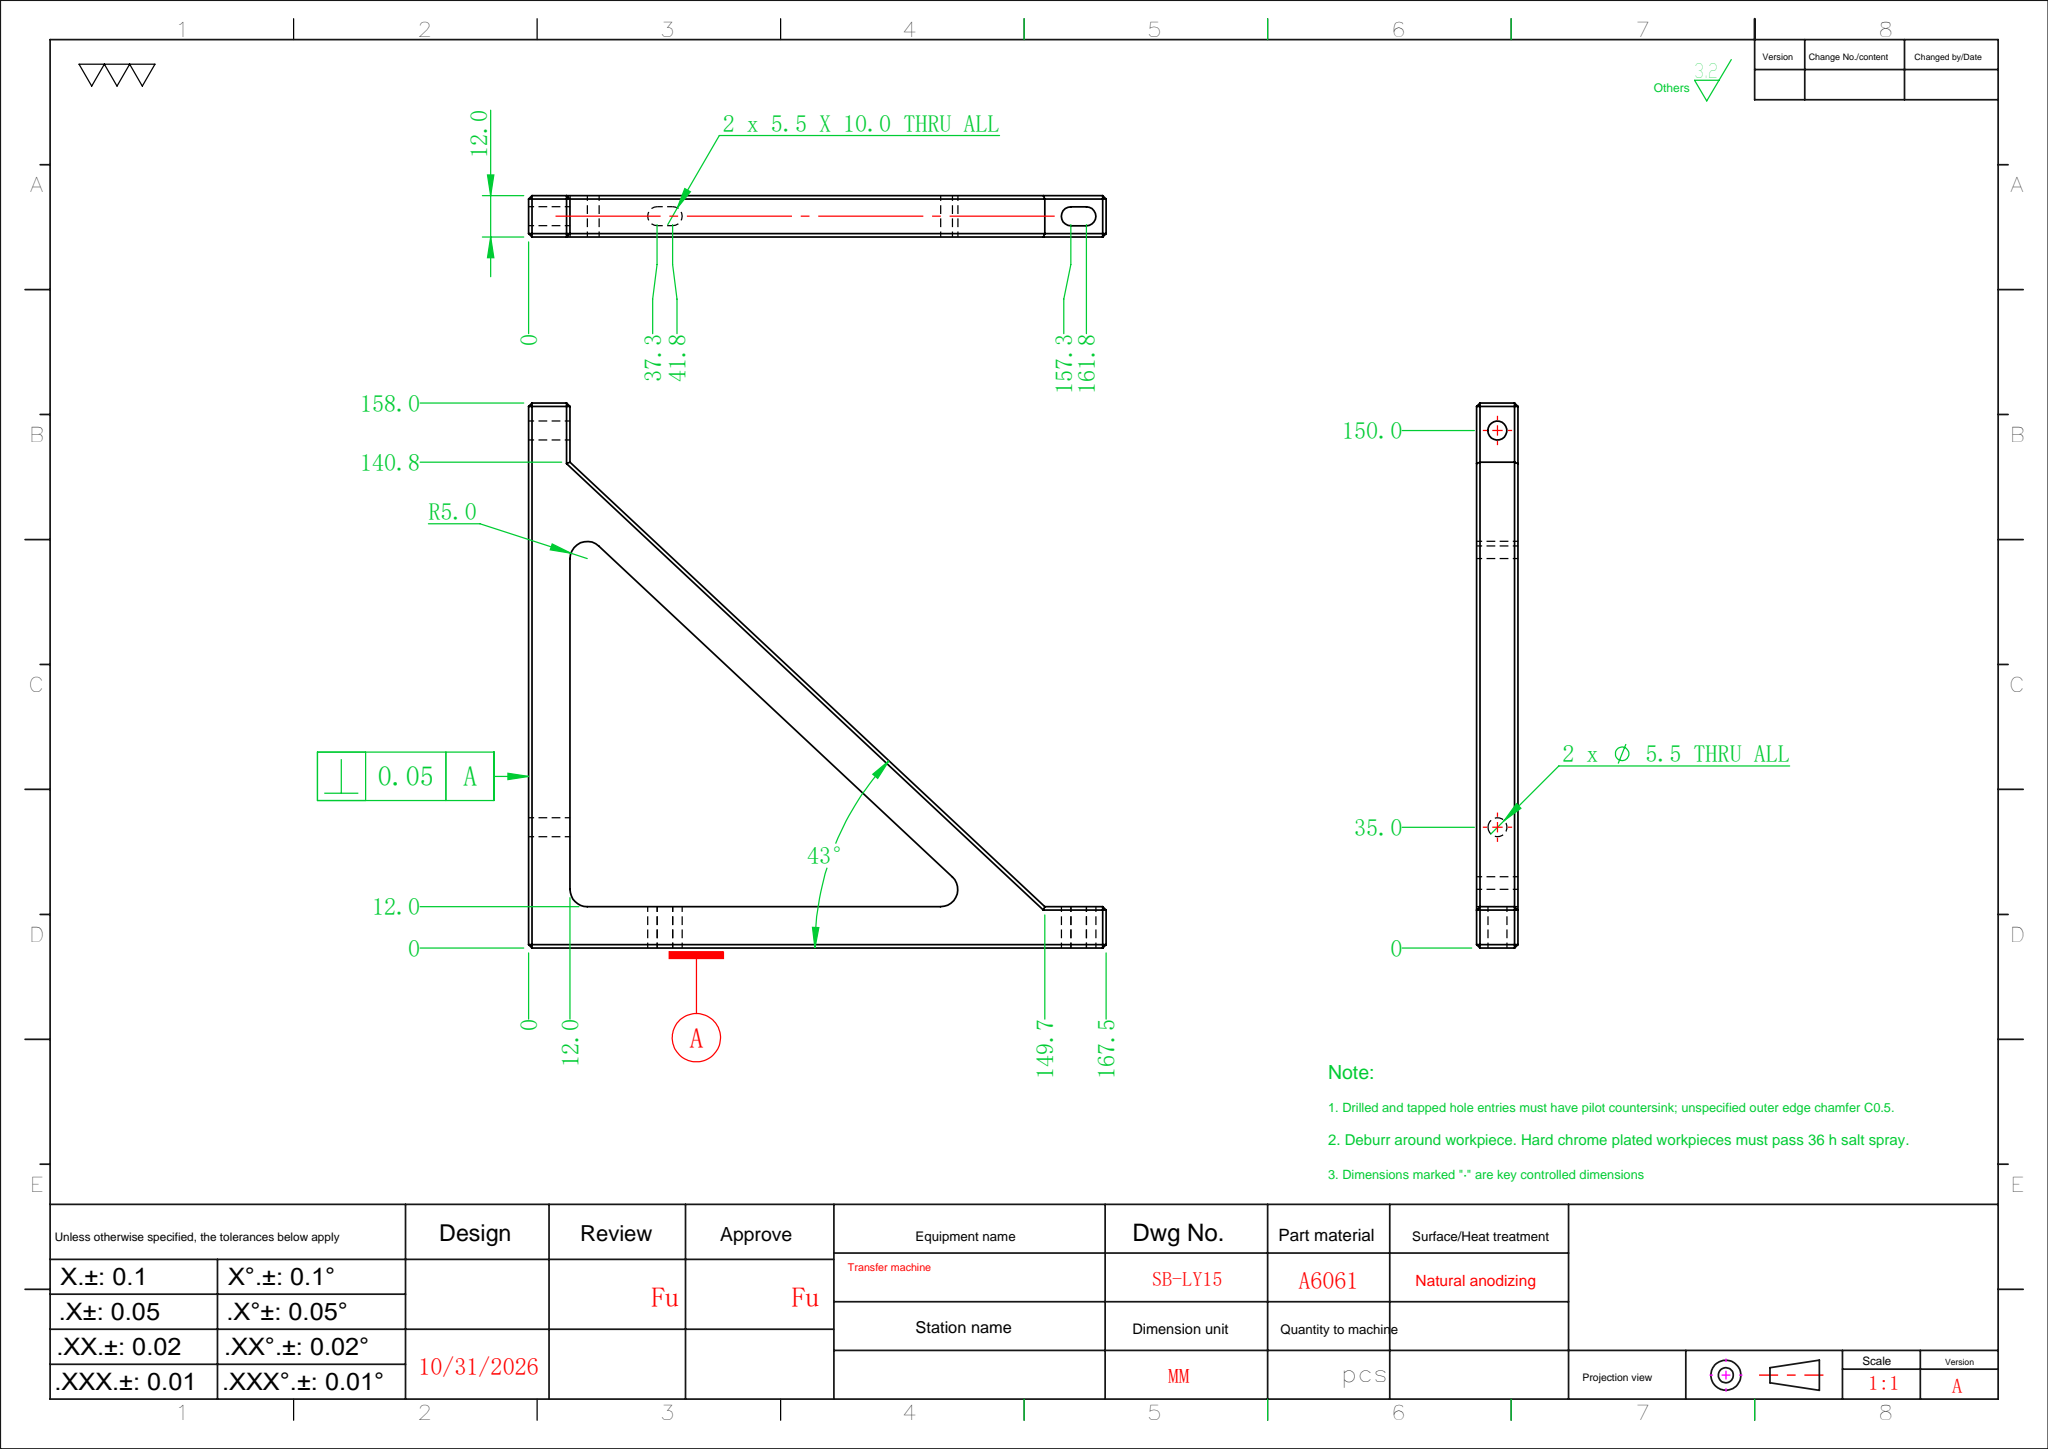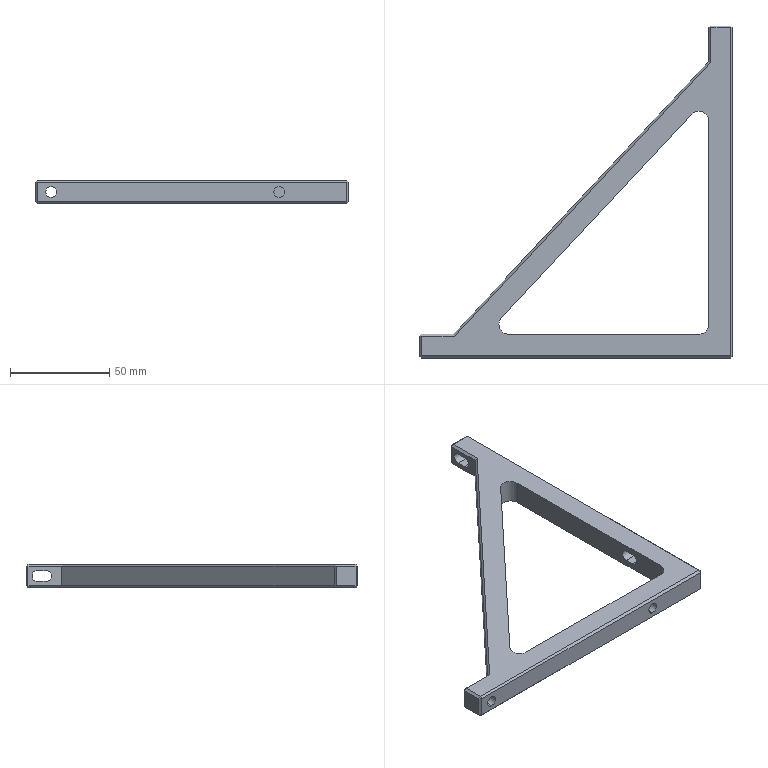Part | SolidWorks | features HoleWzd 2, ICE 2, Chamfer 1, Cut 1, Extrusion 1, Fillet 1 | 1 solid | 57 faces | box 158 x 167.5 x 12 mm | volume 69045 mm3 | plane 45 | cylinder 12 | commonest cylinder face diameters 5.5 x8 10 x4